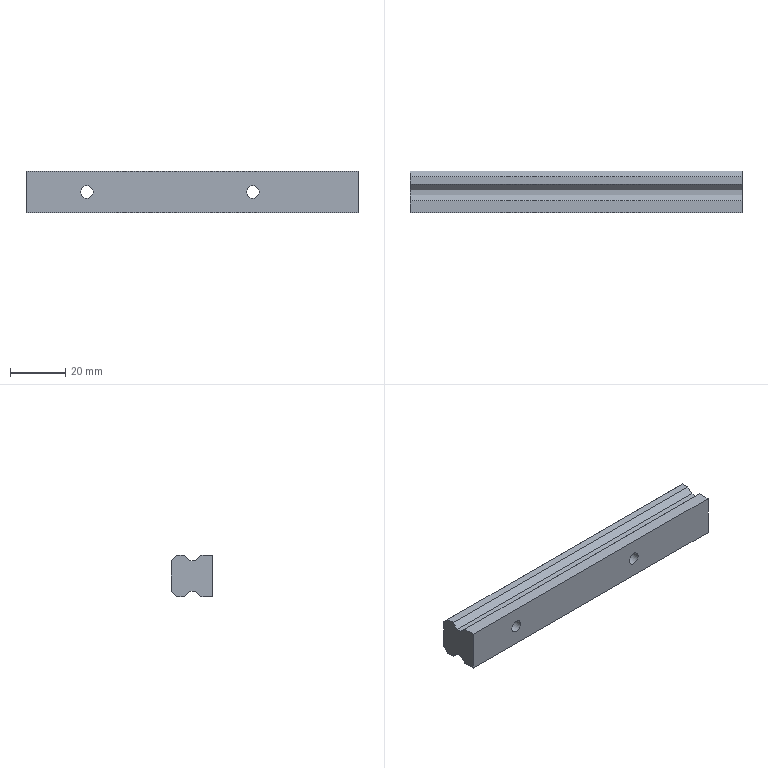Part | NX | features CBORE_HOLE 8, DATUM_CSYS 3, EXTRUDE 2, SKETCH 2, HOLE PACKAGE 1 | 1 solid | 22 faces | box 120 x 15 x 15 mm | volume 23818 mm3 | plane 18 | cylinder 4 | commonest cylinder face diameters 4.5 x2 7.5 x2
STEP:
#1=CARTESIAN_POINT('',(20.,0.,-7.5));
#2=VERTEX_POINT('',#1);
#3=CARTESIAN_POINT('',(-100.,0.,-7.5));
#4=VERTEX_POINT('',#3);
#5=CARTESIAN_POINT('',(20.,0.,-7.5));
#6=DIRECTION('',(-1.,0.,0.));
#7=VECTOR('',#6,1000.);
#8=LINE('',#5,#7);
#9=EDGE_CURVE('',#2,#4,#8,.T.);
#10=ORIENTED_EDGE('',*,*,#9,.T.);
#11=CARTESIAN_POINT('',(-100.,2.,-5.5));
#12=VERTEX_POINT('',#11);
#13=CARTESIAN_POINT('',(-100.,2.,-5.5));
#14=DIRECTION('',(0.,-0.7071,-0.7071));
#15=VECTOR('',#14,1000.);
#16=LINE('',#13,#15);
#17=EDGE_CURVE('',#12,#4,#16,.T.);
#18=ORIENTED_EDGE('',*,*,#17,.F.);
#19=CARTESIAN_POINT('',(20.,2.,-5.5));
#20=VERTEX_POINT('',#19);
#21=CARTESIAN_POINT('',(20.,2.,-5.5));
#22=DIRECTION('',(-1.,0.,0.));
#23=VECTOR('',#22,1000.);
#24=LINE('',#21,#23);
#25=EDGE_CURVE('',#20,#12,#24,.T.);
#26=ORIENTED_EDGE('',*,*,#25,.F.);
#27=CARTESIAN_POINT('',(20.,0.,-7.5));
#28=DIRECTION('',(0.,0.7071,0.7071));
#29=VECTOR('',#28,1000.);
#30=LINE('',#27,#29);
#31=EDGE_CURVE('',#2,#20,#30,.T.);
#32=ORIENTED_EDGE('',*,*,#31,.F.);
#33=EDGE_LOOP('',(#10,#18,#26,#32));
#34=FACE_BOUND('',#33,.T.);
#35=CARTESIAN_POINT('',(20.,0.,-7.5));
#36=DIRECTION('',(0.,-0.7071,0.7071));
#37=DIRECTION('',(0.,-0.7071,-0.7071));
#38=AXIS2_PLACEMENT_3D('',#35,#36,#37);
#39=PLANE('',#38);
#40=ADVANCED_FACE('',(#34),#39,.F.);
#41=ORIENTED_EDGE('',*,*,#25,.T.);
#42=CARTESIAN_POINT('',(-100.,4.,-5.5));
#43=VERTEX_POINT('',#42);
#44=CARTESIAN_POINT('',(-100.,4.,-5.5));
#45=DIRECTION('',(0.,-1.,0.));
#46=VECTOR('',#45,1000.);
#47=LINE('',#44,#46);
#48=EDGE_CURVE('',#43,#12,#47,.T.);
#49=ORIENTED_EDGE('',*,*,#48,.F.);
#50=CARTESIAN_POINT('',(20.,4.,-5.5));
#51=VERTEX_POINT('',#50);
#52=CARTESIAN_POINT('',(20.,4.,-5.5));
#53=DIRECTION('',(-1.,0.,0.));
#54=VECTOR('',#53,1000.);
#55=LINE('',#52,#54);
#56=EDGE_CURVE('',#51,#43,#55,.T.);
#57=ORIENTED_EDGE('',*,*,#56,.F.);
#58=CARTESIAN_POINT('',(20.,2.,-5.5));
#59=DIRECTION('',(0.,1.,0.));
#60=VECTOR('',#59,1000.);
#61=LINE('',#58,#60);
#62=EDGE_CURVE('',#20,#51,#61,.T.);
#63=ORIENTED_EDGE('',*,*,#62,.F.);
#64=EDGE_LOOP('',(#41,#49,#57,#63));
#65=FACE_BOUND('',#64,.T.);
#66=CARTESIAN_POINT('',(20.,2.,-5.5));
#67=DIRECTION('',(0.,0.,1.));
#68=DIRECTION('',(1.,0.,0.));
#69=AXIS2_PLACEMENT_3D('',#66,#67,#68);
#70=PLANE('',#69);
#71=ADVANCED_FACE('',(#65),#70,.F.);
#72=ORIENTED_EDGE('',*,*,#56,.T.);
#73=CARTESIAN_POINT('',(-100.,6.,-7.5));
#74=VERTEX_POINT('',#73);
#75=CARTESIAN_POINT('',(-100.,6.,-7.5));
#76=DIRECTION('',(0.,-0.7071,0.7071));
#77=VECTOR('',#76,1000.);
#78=LINE('',#75,#77);
#79=EDGE_CURVE('',#74,#43,#78,.T.);
#80=ORIENTED_EDGE('',*,*,#79,.F.);
#81=CARTESIAN_POINT('',(20.,6.,-7.5));
#82=VERTEX_POINT('',#81);
#83=CARTESIAN_POINT('',(20.,6.,-7.5));
#84=DIRECTION('',(-1.,0.,0.));
#85=VECTOR('',#84,1000.);
#86=LINE('',#83,#85);
#87=EDGE_CURVE('',#82,#74,#86,.T.);
#88=ORIENTED_EDGE('',*,*,#87,.F.);
#89=CARTESIAN_POINT('',(20.,4.,-5.5));
#90=DIRECTION('',(0.,0.7071,-0.7071));
#91=VECTOR('',#90,1000.);
#92=LINE('',#89,#91);
#93=EDGE_CURVE('',#51,#82,#92,.T.);
#94=ORIENTED_EDGE('',*,*,#93,.F.);
#95=EDGE_LOOP('',(#72,#80,#88,#94));
#96=FACE_BOUND('',#95,.T.);
#97=CARTESIAN_POINT('',(20.,4.,-5.5));
#98=DIRECTION('',(0.,0.7071,0.7071));
#99=DIRECTION('',(0.,-0.7071,0.7071));
#100=AXIS2_PLACEMENT_3D('',#97,#98,#99);
#101=PLANE('',#100);
#102=ADVANCED_FACE('',(#96),#101,.F.);
#103=ORIENTED_EDGE('',*,*,#87,.T.);
#104=CARTESIAN_POINT('',(-100.,8.7,-7.5));
#105=VERTEX_POINT('',#104);
#106=CARTESIAN_POINT('',(-100.,8.7,-7.5));
#107=DIRECTION('',(0.,-1.,0.));
#108=VECTOR('',#107,1000.);
#109=LINE('',#106,#108);
#110=EDGE_CURVE('',#105,#74,#109,.T.);
#111=ORIENTED_EDGE('',*,*,#110,.F.);
#112=CARTESIAN_POINT('',(20.,8.7,-7.5));
#113=VERTEX_POINT('',#112);
#114=CARTESIAN_POINT('',(20.,8.7,-7.5));
#115=DIRECTION('',(-1.,0.,0.));
#116=VECTOR('',#115,1000.);
#117=LINE('',#114,#116);
#118=EDGE_CURVE('',#113,#105,#117,.T.);
#119=ORIENTED_EDGE('',*,*,#118,.F.);
#120=CARTESIAN_POINT('',(20.,6.,-7.5));
#121=DIRECTION('',(0.,1.,0.));
#122=VECTOR('',#121,1000.);
#123=LINE('',#120,#122);
#124=EDGE_CURVE('',#82,#113,#123,.T.);
#125=ORIENTED_EDGE('',*,*,#124,.F.);
#126=EDGE_LOOP('',(#103,#111,#119,#125));
#127=FACE_BOUND('',#126,.T.);
#128=CARTESIAN_POINT('',(20.,6.,-7.5));
#129=DIRECTION('',(0.,0.,1.));
#130=DIRECTION('',(0.,-1.,0.));
#131=AXIS2_PLACEMENT_3D('',#128,#129,#130);
#132=PLANE('',#131);
#133=ADVANCED_FACE('',(#127),#132,.F.);
#134=ORIENTED_EDGE('',*,*,#118,.T.);
#135=CARTESIAN_POINT('',(-100.,10.7,-5.5));
#136=VERTEX_POINT('',#135);
#137=CARTESIAN_POINT('',(-100.,10.7,-5.5));
#138=DIRECTION('',(0.,-0.7071,-0.7071));
#139=VECTOR('',#138,1000.);
#140=LINE('',#137,#139);
#141=EDGE_CURVE('',#136,#105,#140,.T.);
#142=ORIENTED_EDGE('',*,*,#141,.F.);
#143=CARTESIAN_POINT('',(20.,10.7,-5.5));
#144=VERTEX_POINT('',#143);
#145=CARTESIAN_POINT('',(20.,10.7,-5.5));
#146=DIRECTION('',(-1.,0.,0.));
#147=VECTOR('',#146,1000.);
#148=LINE('',#145,#147);
#149=EDGE_CURVE('',#144,#136,#148,.T.);
#150=ORIENTED_EDGE('',*,*,#149,.F.);
#151=CARTESIAN_POINT('',(20.,8.7,-7.5));
#152=DIRECTION('',(0.,0.7071,0.7071));
#153=VECTOR('',#152,1000.);
#154=LINE('',#151,#153);
#155=EDGE_CURVE('',#113,#144,#154,.T.);
#156=ORIENTED_EDGE('',*,*,#155,.F.);
#157=EDGE_LOOP('',(#134,#142,#150,#156));
#158=FACE_BOUND('',#157,.T.);
#159=CARTESIAN_POINT('',(20.,8.7,-7.5));
#160=DIRECTION('',(0.,-0.7071,0.7071));
#161=DIRECTION('',(0.,-0.7071,-0.7071));
#162=AXIS2_PLACEMENT_3D('',#159,#160,#161);
#163=PLANE('',#162);
#164=ADVANCED_FACE('',(#158),#163,.F.);
#165=CARTESIAN_POINT('',(-18.,10.7,-3.75));
#166=VERTEX_POINT('',#165);
#167=CARTESIAN_POINT('',(-18.,10.7,0.));
#168=DIRECTION('',(0.,-1.,0.));
#169=DIRECTION('',(0.,0.,-1.));
#170=AXIS2_PLACEMENT_3D('',#167,#168,#169);
#171=CIRCLE('',#170,3.75);
#172=EDGE_CURVE('',#166,#166,#171,.T.);
#173=ORIENTED_EDGE('',*,*,#172,.T.);
#174=EDGE_LOOP('',(#173));
#175=FACE_BOUND('',#174,.T.);
#176=CARTESIAN_POINT('',(-78.,10.7,-3.75));
#177=VERTEX_POINT('',#176);
#178=CARTESIAN_POINT('',(-78.,10.7,0.));
#179=DIRECTION('',(0.,-1.,0.));
#180=DIRECTION('',(0.,0.,-1.));
#181=AXIS2_PLACEMENT_3D('',#178,#179,#180);
#182=CIRCLE('',#181,3.75);
#183=EDGE_CURVE('',#177,#177,#182,.T.);
#184=ORIENTED_EDGE('',*,*,#183,.T.);
#185=EDGE_LOOP('',(#184));
#186=FACE_BOUND('',#185,.T.);
#187=ORIENTED_EDGE('',*,*,#149,.T.);
#188=CARTESIAN_POINT('',(-100.,10.7,5.5));
#189=VERTEX_POINT('',#188);
#190=CARTESIAN_POINT('',(-100.,10.7,5.5));
#191=DIRECTION('',(0.,0.,-1.));
#192=VECTOR('',#191,1000.);
#193=LINE('',#190,#192);
#194=EDGE_CURVE('',#189,#136,#193,.T.);
#195=ORIENTED_EDGE('',*,*,#194,.F.);
#196=CARTESIAN_POINT('',(20.,10.7,5.5));
#197=VERTEX_POINT('',#196);
#198=CARTESIAN_POINT('',(20.,10.7,5.5));
#199=DIRECTION('',(-1.,0.,0.));
#200=VECTOR('',#199,1000.);
#201=LINE('',#198,#200);
#202=EDGE_CURVE('',#197,#189,#201,.T.);
#203=ORIENTED_EDGE('',*,*,#202,.F.);
#204=CARTESIAN_POINT('',(20.,10.7,-5.5));
#205=DIRECTION('',(0.,0.,1.));
#206=VECTOR('',#205,1000.);
#207=LINE('',#204,#206);
#208=EDGE_CURVE('',#144,#197,#207,.T.);
#209=ORIENTED_EDGE('',*,*,#208,.F.);
#210=EDGE_LOOP('',(#187,#195,#203,#209));
#211=FACE_BOUND('',#210,.T.);
#212=CARTESIAN_POINT('',(20.,10.7,0.));
#213=DIRECTION('',(0.,-1.,0.));
#214=DIRECTION('',(0.,0.,-1.));
#215=AXIS2_PLACEMENT_3D('',#212,#213,#214);
#216=PLANE('',#215);
#217=ADVANCED_FACE('',(#175,#186,#211),#216,.F.);
#218=ORIENTED_EDGE('',*,*,#202,.T.);
#219=CARTESIAN_POINT('',(-100.,8.7,7.5));
#220=VERTEX_POINT('',#219);
#221=CARTESIAN_POINT('',(-100.,8.7,7.5));
#222=DIRECTION('',(0.,0.7071,-0.7071));
#223=VECTOR('',#222,1000.);
#224=LINE('',#221,#223);
#225=EDGE_CURVE('',#220,#189,#224,.T.);
#226=ORIENTED_EDGE('',*,*,#225,.F.);
#227=CARTESIAN_POINT('',(20.,8.7,7.5));
#228=VERTEX_POINT('',#227);
#229=CARTESIAN_POINT('',(20.,8.7,7.5));
#230=DIRECTION('',(-1.,0.,0.));
#231=VECTOR('',#230,1000.);
#232=LINE('',#229,#231);
#233=EDGE_CURVE('',#228,#220,#232,.T.);
#234=ORIENTED_EDGE('',*,*,#233,.F.);
#235=CARTESIAN_POINT('',(20.,10.7,5.5));
#236=DIRECTION('',(0.,-0.7071,0.7071));
#237=VECTOR('',#236,1000.);
#238=LINE('',#235,#237);
#239=EDGE_CURVE('',#197,#228,#238,.T.);
#240=ORIENTED_EDGE('',*,*,#239,.F.);
#241=EDGE_LOOP('',(#218,#226,#234,#240));
#242=FACE_BOUND('',#241,.T.);
#243=CARTESIAN_POINT('',(20.,10.7,5.5));
#244=DIRECTION('',(0.,-0.7071,-0.7071));
#245=DIRECTION('',(0.,0.7071,-0.7071));
#246=AXIS2_PLACEMENT_3D('',#243,#244,#245);
#247=PLANE('',#246);
#248=ADVANCED_FACE('',(#242),#247,.F.);
#249=ORIENTED_EDGE('',*,*,#233,.T.);
#250=CARTESIAN_POINT('',(-100.,6.,7.5));
#251=VERTEX_POINT('',#250);
#252=CARTESIAN_POINT('',(-100.,6.,7.5));
#253=DIRECTION('',(0.,1.,0.));
#254=VECTOR('',#253,1000.);
#255=LINE('',#252,#254);
#256=EDGE_CURVE('',#251,#220,#255,.T.);
#257=ORIENTED_EDGE('',*,*,#256,.F.);
#258=CARTESIAN_POINT('',(20.,6.,7.5));
#259=VERTEX_POINT('',#258);
#260=CARTESIAN_POINT('',(20.,6.,7.5));
#261=DIRECTION('',(-1.,0.,0.));
#262=VECTOR('',#261,1000.);
#263=LINE('',#260,#262);
#264=EDGE_CURVE('',#259,#251,#263,.T.);
#265=ORIENTED_EDGE('',*,*,#264,.F.);
#266=CARTESIAN_POINT('',(20.,8.7,7.5));
#267=DIRECTION('',(0.,-1.,0.));
#268=VECTOR('',#267,1000.);
#269=LINE('',#266,#268);
#270=EDGE_CURVE('',#228,#259,#269,.T.);
#271=ORIENTED_EDGE('',*,*,#270,.F.);
#272=EDGE_LOOP('',(#249,#257,#265,#271));
#273=FACE_BOUND('',#272,.T.);
#274=CARTESIAN_POINT('',(20.,8.7,7.5));
#275=DIRECTION('',(0.,0.,-1.));
#276=DIRECTION('',(0.,1.,0.));
#277=AXIS2_PLACEMENT_3D('',#274,#275,#276);
#278=PLANE('',#277);
#279=ADVANCED_FACE('',(#273),#278,.F.);
#280=ORIENTED_EDGE('',*,*,#264,.T.);
#281=CARTESIAN_POINT('',(-100.,4.,5.5));
#282=VERTEX_POINT('',#281);
#283=CARTESIAN_POINT('',(-100.,4.,5.5));
#284=DIRECTION('',(0.,0.7071,0.7071));
#285=VECTOR('',#284,1000.);
#286=LINE('',#283,#285);
#287=EDGE_CURVE('',#282,#251,#286,.T.);
#288=ORIENTED_EDGE('',*,*,#287,.F.);
#289=CARTESIAN_POINT('',(20.,4.,5.5));
#290=VERTEX_POINT('',#289);
#291=CARTESIAN_POINT('',(20.,4.,5.5));
#292=DIRECTION('',(-1.,0.,0.));
#293=VECTOR('',#292,1000.);
#294=LINE('',#291,#293);
#295=EDGE_CURVE('',#290,#282,#294,.T.);
#296=ORIENTED_EDGE('',*,*,#295,.F.);
#297=CARTESIAN_POINT('',(20.,6.,7.5));
#298=DIRECTION('',(0.,-0.7071,-0.7071));
#299=VECTOR('',#298,1000.);
#300=LINE('',#297,#299);
#301=EDGE_CURVE('',#259,#290,#300,.T.);
#302=ORIENTED_EDGE('',*,*,#301,.F.);
#303=EDGE_LOOP('',(#280,#288,#296,#302));
#304=FACE_BOUND('',#303,.T.);
#305=CARTESIAN_POINT('',(20.,6.,7.5));
#306=DIRECTION('',(0.,0.7071,-0.7071));
#307=DIRECTION('',(0.,0.7071,0.7071));
#308=AXIS2_PLACEMENT_3D('',#305,#306,#307);
#309=PLANE('',#308);
#310=ADVANCED_FACE('',(#304),#309,.F.);
#311=ORIENTED_EDGE('',*,*,#295,.T.);
#312=CARTESIAN_POINT('',(-100.,2.,5.5));
#313=VERTEX_POINT('',#312);
#314=CARTESIAN_POINT('',(-100.,2.,5.5));
#315=DIRECTION('',(0.,1.,0.));
#316=VECTOR('',#315,1000.);
#317=LINE('',#314,#316);
#318=EDGE_CURVE('',#313,#282,#317,.T.);
#319=ORIENTED_EDGE('',*,*,#318,.F.);
#320=CARTESIAN_POINT('',(20.,2.,5.5));
#321=VERTEX_POINT('',#320);
#322=CARTESIAN_POINT('',(20.,2.,5.5));
#323=DIRECTION('',(-1.,0.,0.));
#324=VECTOR('',#323,1000.);
#325=LINE('',#322,#324);
#326=EDGE_CURVE('',#321,#313,#325,.T.);
#327=ORIENTED_EDGE('',*,*,#326,.F.);
#328=CARTESIAN_POINT('',(20.,4.,5.5));
#329=DIRECTION('',(0.,-1.,0.));
#330=VECTOR('',#329,1000.);
#331=LINE('',#328,#330);
#332=EDGE_CURVE('',#290,#321,#331,.T.);
#333=ORIENTED_EDGE('',*,*,#332,.F.);
#334=EDGE_LOOP('',(#311,#319,#327,#333));
#335=FACE_BOUND('',#334,.T.);
#336=CARTESIAN_POINT('',(20.,4.,5.5));
#337=DIRECTION('',(0.,0.,-1.));
#338=DIRECTION('',(-1.,0.,0.));
#339=AXIS2_PLACEMENT_3D('',#336,#337,#338);
#340=PLANE('',#339);
#341=ADVANCED_FACE('',(#335),#340,.F.);
#342=ORIENTED_EDGE('',*,*,#326,.T.);
#343=CARTESIAN_POINT('',(-100.,0.,7.5));
#344=VERTEX_POINT('',#343);
#345=CARTESIAN_POINT('',(-100.,0.,7.5));
#346=DIRECTION('',(0.,0.7071,-0.7071));
#347=VECTOR('',#346,1000.);
#348=LINE('',#345,#347);
#349=EDGE_CURVE('',#344,#313,#348,.T.);
#350=ORIENTED_EDGE('',*,*,#349,.F.);
#351=CARTESIAN_POINT('',(20.,0.,7.5));
#352=VERTEX_POINT('',#351);
#353=CARTESIAN_POINT('',(20.,0.,7.5));
#354=DIRECTION('',(-1.,0.,0.));
#355=VECTOR('',#354,1000.);
#356=LINE('',#353,#355);
#357=EDGE_CURVE('',#352,#344,#356,.T.);
#358=ORIENTED_EDGE('',*,*,#357,.F.);
#359=CARTESIAN_POINT('',(20.,2.,5.5));
#360=DIRECTION('',(0.,-0.7071,0.7071));
#361=VECTOR('',#360,1000.);
#362=LINE('',#359,#361);
#363=EDGE_CURVE('',#321,#352,#362,.T.);
#364=ORIENTED_EDGE('',*,*,#363,.F.);
#365=EDGE_LOOP('',(#342,#350,#358,#364));
#366=FACE_BOUND('',#365,.T.);
#367=CARTESIAN_POINT('',(20.,2.,5.5));
#368=DIRECTION('',(0.,-0.7071,-0.7071));
#369=DIRECTION('',(0.,0.7071,-0.7071));
#370=AXIS2_PLACEMENT_3D('',#367,#368,#369);
#371=PLANE('',#370);
#372=ADVANCED_FACE('',(#366),#371,.F.);
#373=ORIENTED_EDGE('',*,*,#357,.T.);
#374=CARTESIAN_POINT('',(-100.,-4.3,7.5));
#375=VERTEX_POINT('',#374);
#376=CARTESIAN_POINT('',(-100.,-4.3,7.5));
#377=DIRECTION('',(0.,1.,0.));
#378=VECTOR('',#377,1000.);
#379=LINE('',#376,#378);
#380=EDGE_CURVE('',#375,#344,#379,.T.);
#381=ORIENTED_EDGE('',*,*,#380,.F.);
#382=CARTESIAN_POINT('',(20.,-4.3,7.5));
#383=VERTEX_POINT('',#382);
#384=CARTESIAN_POINT('',(20.,-4.3,7.5));
#385=DIRECTION('',(-1.,0.,0.));
#386=VECTOR('',#385,1000.);
#387=LINE('',#384,#386);
#388=EDGE_CURVE('',#383,#375,#387,.T.);
#389=ORIENTED_EDGE('',*,*,#388,.F.);
#390=CARTESIAN_POINT('',(20.,0.,7.5));
#391=DIRECTION('',(0.,-1.,0.));
#392=VECTOR('',#391,1000.);
#393=LINE('',#390,#392);
#394=EDGE_CURVE('',#352,#383,#393,.T.);
#395=ORIENTED_EDGE('',*,*,#394,.F.);
#396=EDGE_LOOP('',(#373,#381,#389,#395));
#397=FACE_BOUND('',#396,.T.);
#398=CARTESIAN_POINT('',(20.,0.,7.5));
#399=DIRECTION('',(0.,0.,-1.));
#400=DIRECTION('',(0.,1.,0.));
#401=AXIS2_PLACEMENT_3D('',#398,#399,#400);
#402=PLANE('',#401);
#403=ADVANCED_FACE('',(#397),#402,.F.);
#404=CARTESIAN_POINT('',(-18.,-4.3,2.25));
#405=VERTEX_POINT('',#404);
#406=CARTESIAN_POINT('',(-18.,-4.3,0.));
#407=DIRECTION('',(0.,1.,0.));
#408=DIRECTION('',(0.,0.,1.));
#409=AXIS2_PLACEMENT_3D('',#406,#407,#408);
#410=CIRCLE('',#409,2.25);
#411=EDGE_CURVE('',#405,#405,#410,.T.);
#412=ORIENTED_EDGE('',*,*,#411,.T.);
#413=EDGE_LOOP('',(#412));
#414=FACE_BOUND('',#413,.T.);
#415=CARTESIAN_POINT('',(-78.,-4.3,2.25));
#416=VERTEX_POINT('',#415);
#417=CARTESIAN_POINT('',(-78.,-4.3,0.));
#418=DIRECTION('',(0.,1.,0.));
#419=DIRECTION('',(0.,0.,1.));
#420=AXIS2_PLACEMENT_3D('',#417,#418,#419);
#421=CIRCLE('',#420,2.25);
#422=EDGE_CURVE('',#416,#416,#421,.T.);
#423=ORIENTED_EDGE('',*,*,#422,.T.);
#424=EDGE_LOOP('',(#423));
#425=FACE_BOUND('',#424,.T.);
#426=ORIENTED_EDGE('',*,*,#388,.T.);
#427=CARTESIAN_POINT('',(-100.,-4.3,-7.5));
#428=VERTEX_POINT('',#427);
#429=CARTESIAN_POINT('',(-100.,-4.3,-7.5));
#430=DIRECTION('',(0.,0.,1.));
#431=VECTOR('',#430,1000.);
#432=LINE('',#429,#431);
#433=EDGE_CURVE('',#428,#375,#432,.T.);
#434=ORIENTED_EDGE('',*,*,#433,.F.);
#435=CARTESIAN_POINT('',(20.,-4.3,-7.5));
#436=VERTEX_POINT('',#435);
#437=CARTESIAN_POINT('',(20.,-4.3,-7.5));
#438=DIRECTION('',(-1.,0.,0.));
#439=VECTOR('',#438,1000.);
#440=LINE('',#437,#439);
#441=EDGE_CURVE('',#436,#428,#440,.T.);
#442=ORIENTED_EDGE('',*,*,#441,.F.);
#443=CARTESIAN_POINT('',(20.,-4.3,7.5));
#444=DIRECTION('',(0.,0.,-1.));
#445=VECTOR('',#444,1000.);
#446=LINE('',#443,#445);
#447=EDGE_CURVE('',#383,#436,#446,.T.);
#448=ORIENTED_EDGE('',*,*,#447,.F.);
#449=EDGE_LOOP('',(#426,#434,#442,#448));
#450=FACE_BOUND('',#449,.T.);
#451=CARTESIAN_POINT('',(20.,-4.3,7.5));
#452=DIRECTION('',(0.,1.,0.));
#453=DIRECTION('',(0.,0.,1.));
#454=AXIS2_PLACEMENT_3D('',#451,#452,#453);
#455=PLANE('',#454);
#456=ADVANCED_FACE('',(#414,#425,#450),#455,.F.);
#457=ORIENTED_EDGE('',*,*,#441,.T.);
#458=CARTESIAN_POINT('',(-100.,0.,-7.5));
#459=DIRECTION('',(0.,-1.,0.));
#460=VECTOR('',#459,1000.);
#461=LINE('',#458,#460);
#462=EDGE_CURVE('',#4,#428,#461,.T.);
#463=ORIENTED_EDGE('',*,*,#462,.F.);
#464=ORIENTED_EDGE('',*,*,#9,.F.);
#465=CARTESIAN_POINT('',(20.,-4.3,-7.5));
#466=DIRECTION('',(0.,1.,0.));
#467=VECTOR('',#466,1000.);
#468=LINE('',#465,#467);
#469=EDGE_CURVE('',#436,#2,#468,.T.);
#470=ORIENTED_EDGE('',*,*,#469,.F.);
#471=EDGE_LOOP('',(#457,#463,#464,#470));
#472=FACE_BOUND('',#471,.T.);
#473=CARTESIAN_POINT('',(20.,-4.3,-7.5));
#474=DIRECTION('',(0.,0.,1.));
#475=DIRECTION('',(0.,-1.,0.));
#476=AXIS2_PLACEMENT_3D('',#473,#474,#475);
#477=PLANE('',#476);
#478=ADVANCED_FACE('',(#472),#477,.F.);
#479=ORIENTED_EDGE('',*,*,#31,.T.);
#480=ORIENTED_EDGE('',*,*,#62,.T.);
#481=ORIENTED_EDGE('',*,*,#93,.T.);
#482=ORIENTED_EDGE('',*,*,#124,.T.);
#483=ORIENTED_EDGE('',*,*,#155,.T.);
#484=ORIENTED_EDGE('',*,*,#208,.T.);
#485=ORIENTED_EDGE('',*,*,#239,.T.);
#486=ORIENTED_EDGE('',*,*,#270,.T.);
#487=ORIENTED_EDGE('',*,*,#301,.T.);
#488=ORIENTED_EDGE('',*,*,#332,.T.);
#489=ORIENTED_EDGE('',*,*,#363,.T.);
#490=ORIENTED_EDGE('',*,*,#394,.T.);
#491=ORIENTED_EDGE('',*,*,#447,.T.);
#492=ORIENTED_EDGE('',*,*,#469,.T.);
#493=EDGE_LOOP('',(#479,#480,#481,#482,#483,#484,#485,#486,#487,#488,#489,#490,#491,#492));
#494=FACE_BOUND('',#493,.T.);
#495=CARTESIAN_POINT('',(20.,0.,0.));
#496=DIRECTION('',(-1.,0.,0.));
#497=DIRECTION('',(0.,0.,1.));
#498=AXIS2_PLACEMENT_3D('',#495,#496,#497);
#499=PLANE('',#498);
#500=ADVANCED_FACE('',(#494),#499,.F.);
#501=CARTESIAN_POINT('',(-78.,5.3,-2.25));
#502=VERTEX_POINT('',#501);
#503=CARTESIAN_POINT('',(-78.,5.3,0.));
#504=DIRECTION('',(0.,-1.,0.));
#505=DIRECTION('',(0.,0.,-1.));
#506=AXIS2_PLACEMENT_3D('',#503,#504,#505);
#507=CIRCLE('',#506,2.25);
#508=EDGE_CURVE('',#502,#502,#507,.F.);
#509=ORIENTED_EDGE('',*,*,#508,.T.);
#510=EDGE_LOOP('',(#509));
#511=FACE_BOUND('',#510,.T.);
#512=ORIENTED_EDGE('',*,*,#422,.F.);
#513=EDGE_LOOP('',(#512));
#514=FACE_BOUND('',#513,.T.);
#515=CARTESIAN_POINT('',(-78.,-38.375,0.));
#516=DIRECTION('',(0.,-1.,0.));
#517=DIRECTION('',(0.,0.,-1.));
#518=AXIS2_PLACEMENT_3D('',#515,#516,#517);
#519=CYLINDRICAL_SURFACE('',#518,2.25);
#520=ADVANCED_FACE('',(#511,#514),#519,.F.);
#521=ORIENTED_EDGE('',*,*,#508,.F.);
#522=EDGE_LOOP('',(#521));
#523=FACE_BOUND('',#522,.T.);
#524=CARTESIAN_POINT('',(-78.,5.3,-3.75));
#525=VERTEX_POINT('',#524);
#526=CARTESIAN_POINT('',(-78.,5.3,0.));
#527=DIRECTION('',(0.,-1.,0.));
#528=DIRECTION('',(0.,0.,-1.));
#529=AXIS2_PLACEMENT_3D('',#526,#527,#528);
#530=CIRCLE('',#529,3.75);
#531=EDGE_CURVE('',#525,#525,#530,.F.);
#532=ORIENTED_EDGE('',*,*,#531,.T.);
#533=EDGE_LOOP('',(#532));
#534=FACE_BOUND('',#533,.T.);
#535=CARTESIAN_POINT('',(-78.,5.3,0.));
#536=DIRECTION('',(0.,-1.,0.));
#537=DIRECTION('',(0.,0.,-1.));
#538=AXIS2_PLACEMENT_3D('',#535,#536,#537);
#539=PLANE('',#538);
#540=ADVANCED_FACE('',(#523,#534),#539,.F.);
#541=ORIENTED_EDGE('',*,*,#531,.F.);
#542=EDGE_LOOP('',(#541));
#543=FACE_BOUND('',#542,.T.);
#544=ORIENTED_EDGE('',*,*,#183,.F.);
#545=EDGE_LOOP('',(#544));
#546=FACE_BOUND('',#545,.T.);
#547=CARTESIAN_POINT('',(-78.,10.7,0.));
#548=DIRECTION('',(0.,-1.,0.));
#549=DIRECTION('',(0.,0.,-1.));
#550=AXIS2_PLACEMENT_3D('',#547,#548,#549);
#551=CYLINDRICAL_SURFACE('',#550,3.75);
#552=ADVANCED_FACE('',(#543,#546),#551,.F.);
#553=CARTESIAN_POINT('',(-18.,5.3,-2.25));
#554=VERTEX_POINT('',#553);
#555=CARTESIAN_POINT('',(-18.,5.3,0.));
#556=DIRECTION('',(0.,-1.,0.));
#557=DIRECTION('',(0.,0.,-1.));
#558=AXIS2_PLACEMENT_3D('',#555,#556,#557);
#559=CIRCLE('',#558,2.25);
#560=EDGE_CURVE('',#554,#554,#559,.F.);
#561=ORIENTED_EDGE('',*,*,#560,.T.);
#562=EDGE_LOOP('',(#561));
#563=FACE_BOUND('',#562,.T.);
#564=ORIENTED_EDGE('',*,*,#411,.F.);
#565=EDGE_LOOP('',(#564));
#566=FACE_BOUND('',#565,.T.);
#567=CARTESIAN_POINT('',(-18.,-55.182,0.));
#568=DIRECTION('',(0.,-1.,0.));
#569=DIRECTION('',(0.,0.,-1.));
#570=AXIS2_PLACEMENT_3D('',#567,#568,#569);
#571=CYLINDRICAL_SURFACE('',#570,2.25);
#572=ADVANCED_FACE('',(#563,#566),#571,.F.);
#573=ORIENTED_EDGE('',*,*,#560,.F.);
#574=EDGE_LOOP('',(#573));
#575=FACE_BOUND('',#574,.T.);
#576=CARTESIAN_POINT('',(-18.,5.3,-3.75));
#577=VERTEX_POINT('',#576);
#578=CARTESIAN_POINT('',(-18.,5.3,0.));
#579=DIRECTION('',(0.,-1.,0.));
#580=DIRECTION('',(0.,0.,-1.));
#581=AXIS2_PLACEMENT_3D('',#578,#579,#580);
#582=CIRCLE('',#581,3.75);
#583=EDGE_CURVE('',#577,#577,#582,.F.);
#584=ORIENTED_EDGE('',*,*,#583,.T.);
#585=EDGE_LOOP('',(#584));
#586=FACE_BOUND('',#585,.T.);
#587=CARTESIAN_POINT('',(-18.,5.3,0.));
#588=DIRECTION('',(0.,-1.,0.));
#589=DIRECTION('',(0.,0.,-1.));
#590=AXIS2_PLACEMENT_3D('',#587,#588,#589);
#591=PLANE('',#590);
#592=ADVANCED_FACE('',(#575,#586),#591,.F.);
#593=ORIENTED_EDGE('',*,*,#583,.F.);
#594=EDGE_LOOP('',(#593));
#595=FACE_BOUND('',#594,.T.);
#596=ORIENTED_EDGE('',*,*,#172,.F.);
#597=EDGE_LOOP('',(#596));
#598=FACE_BOUND('',#597,.T.);
#599=CARTESIAN_POINT('',(-18.,10.7,0.));
#600=DIRECTION('',(0.,-1.,0.));
#601=DIRECTION('',(0.,0.,-1.));
#602=AXIS2_PLACEMENT_3D('',#599,#600,#601);
#603=CYLINDRICAL_SURFACE('',#602,3.75);
#604=ADVANCED_FACE('',(#595,#598),#603,.F.);
#605=ORIENTED_EDGE('',*,*,#433,.T.);
#606=ORIENTED_EDGE('',*,*,#380,.T.);
#607=ORIENTED_EDGE('',*,*,#349,.T.);
#608=ORIENTED_EDGE('',*,*,#318,.T.);
#609=ORIENTED_EDGE('',*,*,#287,.T.);
#610=ORIENTED_EDGE('',*,*,#256,.T.);
#611=ORIENTED_EDGE('',*,*,#225,.T.);
#612=ORIENTED_EDGE('',*,*,#194,.T.);
#613=ORIENTED_EDGE('',*,*,#141,.T.);
#614=ORIENTED_EDGE('',*,*,#110,.T.);
#615=ORIENTED_EDGE('',*,*,#79,.T.);
#616=ORIENTED_EDGE('',*,*,#48,.T.);
#617=ORIENTED_EDGE('',*,*,#17,.T.);
#618=ORIENTED_EDGE('',*,*,#462,.T.);
#619=EDGE_LOOP('',(#605,#606,#607,#608,#609,#610,#611,#612,#613,#614,#615,#616,#617,#618));
#620=FACE_BOUND('',#619,.T.);
#621=CARTESIAN_POINT('',(-100.,0.,0.));
#622=DIRECTION('',(-1.,0.,0.));
#623=DIRECTION('',(0.,0.,1.));
#624=AXIS2_PLACEMENT_3D('',#621,#622,#623);
#625=PLANE('',#624);
#626=ADVANCED_FACE('',(#620),#625,.T.);
#627=CLOSED_SHELL('',(#40,#71,#102,#133,#164,#217,#248,#279,#310,#341,#372,#403,#456,#478,#500,#520,#540,#552,#572,#592,#604,#626));
#628=MANIFOLD_SOLID_BREP('',#627);
#629=(LENGTH_UNIT()NAMED_UNIT(*)SI_UNIT(.MILLI.,.METRE.));
#630=UNCERTAINTY_MEASURE_WITH_UNIT(LENGTH_MEASURE(0.00001),#629,'','');
#631=(NAMED_UNIT(*)PLANE_ANGLE_UNIT()SI_UNIT($,.RADIAN.));
#632=(NAMED_UNIT(*)SI_UNIT($,.STERADIAN.)SOLID_ANGLE_UNIT());
#633=(GEOMETRIC_REPRESENTATION_CONTEXT(3)GLOBAL_UNCERTAINTY_ASSIGNED_CONTEXT((#630))GLOBAL_UNIT_ASSIGNED_CONTEXT((#629,#631,#632))REPRESENTATION_CONTEXT('',''));
#634=ADVANCED_BREP_SHAPE_REPRESENTATION('',(#628),#633);